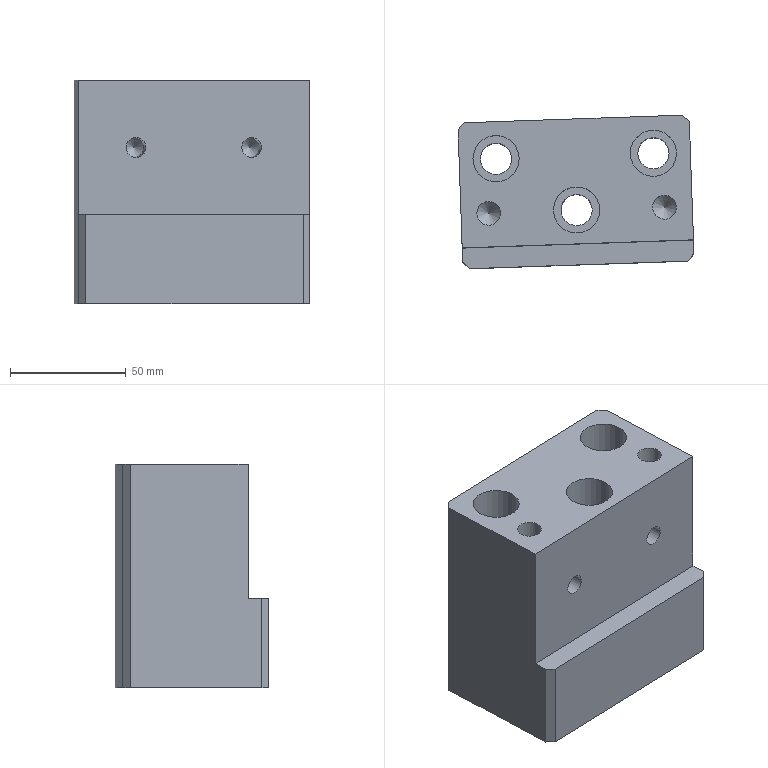Part | NX | features LB-14 2 | 1 solid | 29 faces | box 101.928 x 66.242 x 96.5 mm | volume 491089 mm3 | plane 15 | cylinder 10 | cone 4 | commonest cylinder face diameters 13.5 x3 20 x3 8.506 x2 10.3 x2
STEP:
#1=CARTESIAN_POINT('',(3839.924,-622.872,788.716));
#2=VERTEX_POINT('',#1);
#3=CARTESIAN_POINT('',(3833.174,-622.872,788.716));
#4=DIRECTION('',(-0.000000002,0.,1.));
#5=DIRECTION('',(1.,0.,0.000000002));
#6=AXIS2_PLACEMENT_3D('',#3,#4,#5);
#7=CIRCLE('',#6,6.75);
#8=EDGE_CURVE('',#2,#2,#7,.F.);
#9=ORIENTED_EDGE('',*,*,#8,.F.);
#10=EDGE_LOOP('',(#9));
#11=FACE_BOUND('',#10,.T.);
#12=CARTESIAN_POINT('',(3850.699,-666.287,788.716));
#13=VERTEX_POINT('',#12);
#14=CARTESIAN_POINT('',(3848.71,-609.321,788.716));
#15=VERTEX_POINT('',#14);
#16=CARTESIAN_POINT('',(3848.745,-610.321,788.716));
#17=DIRECTION('',(-0.0349,0.9994,0.));
#18=VECTOR('',#17,1000.);
#19=LINE('',#16,#18);
#20=EDGE_CURVE('',#13,#15,#19,.T.);
#21=ORIENTED_EDGE('',*,*,#20,.F.);
#22=CARTESIAN_POINT('',(3847.806,-669.389,788.716));
#23=VERTEX_POINT('',#22);
#24=CARTESIAN_POINT('',(3830.445,-688.007,788.716));
#25=DIRECTION('',(-0.682,-0.7314,-0.000000001));
#26=VECTOR('',#25,1000.);
#27=LINE('',#24,#26);
#28=EDGE_CURVE('',#23,#13,#27,.F.);
#29=ORIENTED_EDGE('',*,*,#28,.F.);
#30=CARTESIAN_POINT('',(3753.863,-672.67,788.716));
#31=VERTEX_POINT('',#30);
#32=CARTESIAN_POINT('',(3752.864,-672.705,788.716));
#33=DIRECTION('',(0.9994,0.0349,0.000000002));
#34=VECTOR('',#33,1000.);
#35=LINE('',#32,#34);
#36=EDGE_CURVE('',#31,#23,#35,.T.);
#37=ORIENTED_EDGE('',*,*,#36,.F.);
#38=CARTESIAN_POINT('',(3750.76,-669.776,788.716));
#39=VERTEX_POINT('',#38);
#40=CARTESIAN_POINT('',(3722.835,-643.735,788.716));
#41=DIRECTION('',(-0.7314,0.682,-0.000000001));
#42=VECTOR('',#41,1000.);
#43=LINE('',#40,#42);
#44=EDGE_CURVE('',#39,#31,#43,.F.);
#45=ORIENTED_EDGE('',*,*,#44,.F.);
#46=CARTESIAN_POINT('',(3748.771,-612.811,788.716));
#47=VERTEX_POINT('',#46);
#48=CARTESIAN_POINT('',(3748.806,-613.81,788.716));
#49=DIRECTION('',(0.0349,-0.9994,0.));
#50=VECTOR('',#49,1000.);
#51=LINE('',#48,#50);
#52=EDGE_CURVE('',#47,#39,#51,.T.);
#53=ORIENTED_EDGE('',*,*,#52,.F.);
#54=CARTESIAN_POINT('',(3751.665,-609.708,788.716));
#55=VERTEX_POINT('',#54);
#56=CARTESIAN_POINT('',(3749.254,-612.294,788.716));
#57=DIRECTION('',(0.682,0.7314,0.000000001));
#58=VECTOR('',#57,1000.);
#59=LINE('',#56,#58);
#60=EDGE_CURVE('',#55,#47,#59,.F.);
#61=ORIENTED_EDGE('',*,*,#60,.F.);
#62=CARTESIAN_POINT('',(3845.608,-606.428,788.716));
#63=VERTEX_POINT('',#62);
#64=CARTESIAN_POINT('',(3750.665,-609.743,788.716));
#65=DIRECTION('',(-0.9994,-0.0349,-0.000000002));
#66=VECTOR('',#65,1000.);
#67=LINE('',#64,#66);
#68=EDGE_CURVE('',#63,#55,#67,.T.);
#69=ORIENTED_EDGE('',*,*,#68,.F.);
#70=CARTESIAN_POINT('',(3798.548,-562.543,788.716));
#71=DIRECTION('',(0.7314,-0.682,0.000000001));
#72=VECTOR('',#71,1000.);
#73=LINE('',#70,#72);
#74=EDGE_CURVE('',#15,#63,#73,.F.);
#75=ORIENTED_EDGE('',*,*,#74,.F.);
#76=EDGE_LOOP('',(#21,#29,#37,#45,#53,#61,#69,#75));
#77=FACE_BOUND('',#76,.T.);
#78=CARTESIAN_POINT('',(3806.76,-647.401,788.716));
#79=VERTEX_POINT('',#78);
#80=CARTESIAN_POINT('',(3800.01,-647.401,788.716));
#81=DIRECTION('',(-0.000000002,0.,1.));
#82=DIRECTION('',(1.,0.,0.000000002));
#83=AXIS2_PLACEMENT_3D('',#80,#81,#82);
#84=CIRCLE('',#83,6.75);
#85=EDGE_CURVE('',#79,#79,#84,.F.);
#86=ORIENTED_EDGE('',*,*,#85,.F.);
#87=EDGE_LOOP('',(#86));
#88=FACE_BOUND('',#87,.T.);
#89=CARTESIAN_POINT('',(3771.965,-625.245,788.716));
#90=VERTEX_POINT('',#89);
#91=CARTESIAN_POINT('',(3765.215,-625.245,788.716));
#92=DIRECTION('',(-0.000000002,0.,1.));
#93=DIRECTION('',(1.,0.,0.000000002));
#94=AXIS2_PLACEMENT_3D('',#91,#92,#93);
#95=CIRCLE('',#94,6.75);
#96=EDGE_CURVE('',#90,#90,#95,.F.);
#97=ORIENTED_EDGE('',*,*,#96,.F.);
#98=EDGE_LOOP('',(#97));
#99=FACE_BOUND('',#98,.T.);
#100=CARTESIAN_POINT('',(3750.805,-613.741,788.716));
#101=DIRECTION('',(-0.000000002,0.,1.));
#102=DIRECTION('',(0.9994,0.0349,0.000000002));
#103=AXIS2_PLACEMENT_3D('',#100,#101,#102);
#104=PLANE('',#103);
#105=ADVANCED_FACE('',(#11,#77,#88,#99),#104,.F.);
#106=CARTESIAN_POINT('',(3810.01,-647.401,885.216));
#107=VERTEX_POINT('',#106);
#108=CARTESIAN_POINT('',(3800.01,-647.401,885.216));
#109=DIRECTION('',(0.,0.,1.));
#110=DIRECTION('',(1.,0.,0.));
#111=AXIS2_PLACEMENT_3D('',#108,#109,#110);
#112=CIRCLE('',#111,10.);
#113=EDGE_CURVE('',#107,#107,#112,.T.);
#114=ORIENTED_EDGE('',*,*,#113,.F.);
#115=EDGE_LOOP('',(#114));
#116=FACE_BOUND('',#115,.T.);
#117=CARTESIAN_POINT('',(3767.185,-648.69,885.216));
#118=VERTEX_POINT('',#117);
#119=CARTESIAN_POINT('',(3762.038,-648.87,885.216));
#120=DIRECTION('',(0.000000002,0.,-1.));
#121=DIRECTION('',(0.9994,0.0349,0.000000002));
#122=AXIS2_PLACEMENT_3D('',#119,#120,#121);
#123=CIRCLE('',#122,5.15);
#124=EDGE_CURVE('',#118,#118,#123,.T.);
#125=ORIENTED_EDGE('',*,*,#124,.T.);
#126=EDGE_LOOP('',(#125));
#127=FACE_BOUND('',#126,.T.);
#128=CARTESIAN_POINT('',(3843.138,-646.038,885.216));
#129=VERTEX_POINT('',#128);
#130=CARTESIAN_POINT('',(3837.991,-646.218,885.216));
#131=DIRECTION('',(0.000000002,0.,-1.));
#132=DIRECTION('',(0.9994,0.0349,0.000000002));
#133=AXIS2_PLACEMENT_3D('',#130,#131,#132);
#134=CIRCLE('',#133,5.15);
#135=EDGE_CURVE('',#129,#129,#134,.T.);
#136=ORIENTED_EDGE('',*,*,#135,.T.);
#137=EDGE_LOOP('',(#136));
#138=FACE_BOUND('',#137,.T.);
#139=CARTESIAN_POINT('',(3748.771,-612.811,885.216));
#140=VERTEX_POINT('',#139);
#141=CARTESIAN_POINT('',(3750.551,-663.78,885.216));
#142=VERTEX_POINT('',#141);
#143=CARTESIAN_POINT('',(3748.387,-601.818,885.216));
#144=DIRECTION('',(0.0349,-0.9994,0.));
#145=VECTOR('',#144,1000.);
#146=LINE('',#143,#145);
#147=EDGE_CURVE('',#140,#142,#146,.T.);
#148=ORIENTED_EDGE('',*,*,#147,.T.);
#149=CARTESIAN_POINT('',(3850.49,-660.29,885.216));
#150=VERTEX_POINT('',#149);
#151=CARTESIAN_POINT('',(3983.632,-655.641,885.216));
#152=DIRECTION('',(-0.9994,-0.0349,-0.000000002));
#153=VECTOR('',#152,1000.);
#154=LINE('',#151,#153);
#155=EDGE_CURVE('',#150,#142,#154,.T.);
#156=ORIENTED_EDGE('',*,*,#155,.F.);
#157=CARTESIAN_POINT('',(3848.71,-609.321,885.216));
#158=VERTEX_POINT('',#157);
#159=CARTESIAN_POINT('',(3848.745,-610.321,885.216));
#160=DIRECTION('',(0.0349,-0.9994,0.));
#161=VECTOR('',#160,1000.);
#162=LINE('',#159,#161);
#163=EDGE_CURVE('',#158,#150,#162,.T.);
#164=ORIENTED_EDGE('',*,*,#163,.F.);
#165=CARTESIAN_POINT('',(3845.608,-606.428,885.216));
#166=VERTEX_POINT('',#165);
#167=CARTESIAN_POINT('',(3798.548,-562.543,885.216));
#168=DIRECTION('',(-0.7314,0.682,-0.000000001));
#169=VECTOR('',#168,1000.);
#170=LINE('',#167,#169);
#171=EDGE_CURVE('',#166,#158,#170,.F.);
#172=ORIENTED_EDGE('',*,*,#171,.F.);
#173=CARTESIAN_POINT('',(3751.665,-609.708,885.216));
#174=VERTEX_POINT('',#173);
#175=CARTESIAN_POINT('',(3813.627,-607.545,885.216));
#176=DIRECTION('',(-0.9994,-0.0349,-0.000000002));
#177=VECTOR('',#176,1000.);
#178=LINE('',#175,#177);
#179=EDGE_CURVE('',#166,#174,#178,.T.);
#180=ORIENTED_EDGE('',*,*,#179,.T.);
#181=CARTESIAN_POINT('',(3749.254,-612.294,885.216));
#182=DIRECTION('',(-0.682,-0.7314,-0.000000001));
#183=VECTOR('',#182,1000.);
#184=LINE('',#181,#183);
#185=EDGE_CURVE('',#140,#174,#184,.F.);
#186=ORIENTED_EDGE('',*,*,#185,.F.);
#187=EDGE_LOOP('',(#148,#156,#164,#172,#180,#186));
#188=FACE_BOUND('',#187,.T.);
#189=CARTESIAN_POINT('',(3775.215,-625.245,885.216));
#190=VERTEX_POINT('',#189);
#191=CARTESIAN_POINT('',(3765.215,-625.245,885.216));
#192=DIRECTION('',(0.,0.,1.));
#193=DIRECTION('',(1.,0.,0.));
#194=AXIS2_PLACEMENT_3D('',#191,#192,#193);
#195=CIRCLE('',#194,10.);
#196=EDGE_CURVE('',#190,#190,#195,.T.);
#197=ORIENTED_EDGE('',*,*,#196,.F.);
#198=EDGE_LOOP('',(#197));
#199=FACE_BOUND('',#198,.T.);
#200=CARTESIAN_POINT('',(3843.174,-622.872,885.216));
#201=VERTEX_POINT('',#200);
#202=CARTESIAN_POINT('',(3833.174,-622.872,885.216));
#203=DIRECTION('',(0.,0.,1.));
#204=DIRECTION('',(1.,0.,0.));
#205=AXIS2_PLACEMENT_3D('',#202,#203,#204);
#206=CIRCLE('',#205,10.);
#207=EDGE_CURVE('',#201,#201,#206,.T.);
#208=ORIENTED_EDGE('',*,*,#207,.F.);
#209=EDGE_LOOP('',(#208));
#210=FACE_BOUND('',#209,.T.);
#211=CARTESIAN_POINT('',(3750.805,-613.741,885.216));
#212=DIRECTION('',(-0.000000002,0.,1.));
#213=DIRECTION('',(0.9994,0.0349,0.000000002));
#214=AXIS2_PLACEMENT_3D('',#211,#212,#213);
#215=PLANE('',#214);
#216=ADVANCED_FACE('',(#116,#127,#138,#188,#199,#210),#215,.T.);
#217=CARTESIAN_POINT('',(3775.536,-662.907,851.963));
#218=VERTEX_POINT('',#217);
#219=CARTESIAN_POINT('',(3775.536,-662.907,856.216));
#220=DIRECTION('',(0.0349,-0.9994,0.));
#221=DIRECTION('',(0.000000002,0.,-1.));
#222=AXIS2_PLACEMENT_3D('',#219,#220,#221);
#223=CIRCLE('',#222,4.253);
#224=EDGE_CURVE('',#218,#218,#223,.T.);
#225=ORIENTED_EDGE('',*,*,#224,.T.);
#226=EDGE_LOOP('',(#225));
#227=FACE_BOUND('',#226,.T.);
#228=CARTESIAN_POINT('',(3774.637,-637.176,860.469));
#229=VERTEX_POINT('',#228);
#230=CARTESIAN_POINT('',(3774.637,-637.176,856.216));
#231=DIRECTION('',(-0.0349,0.9994,0.));
#232=DIRECTION('',(-0.000000002,0.,1.));
#233=AXIS2_PLACEMENT_3D('',#230,#231,#232);
#234=CIRCLE('',#233,4.253);
#235=EDGE_CURVE('',#229,#229,#234,.F.);
#236=ORIENTED_EDGE('',*,*,#235,.F.);
#237=EDGE_LOOP('',(#236));
#238=FACE_BOUND('',#237,.T.);
#239=CARTESIAN_POINT('',(3775.536,-662.907,856.216));
#240=DIRECTION('',(-0.0349,0.9994,0.));
#241=DIRECTION('',(-0.9994,-0.0349,-0.000000002));
#242=AXIS2_PLACEMENT_3D('',#239,#240,#241);
#243=CYLINDRICAL_SURFACE('',#242,4.253);
#244=ADVANCED_FACE('',(#227,#238),#243,.F.);
#245=CARTESIAN_POINT('',(3825.505,-661.163,851.963));
#246=VERTEX_POINT('',#245);
#247=CARTESIAN_POINT('',(3825.505,-661.163,856.216));
#248=DIRECTION('',(0.0349,-0.9994,0.));
#249=DIRECTION('',(0.000000002,0.,-1.));
#250=AXIS2_PLACEMENT_3D('',#247,#248,#249);
#251=CIRCLE('',#250,4.253);
#252=EDGE_CURVE('',#246,#246,#251,.T.);
#253=ORIENTED_EDGE('',*,*,#252,.T.);
#254=EDGE_LOOP('',(#253));
#255=FACE_BOUND('',#254,.T.);
#256=CARTESIAN_POINT('',(3824.607,-635.431,860.469));
#257=VERTEX_POINT('',#256);
#258=CARTESIAN_POINT('',(3824.607,-635.431,856.216));
#259=DIRECTION('',(-0.0349,0.9994,0.));
#260=DIRECTION('',(-0.000000002,0.,1.));
#261=AXIS2_PLACEMENT_3D('',#258,#259,#260);
#262=CIRCLE('',#261,4.253);
#263=EDGE_CURVE('',#257,#257,#262,.F.);
#264=ORIENTED_EDGE('',*,*,#263,.F.);
#265=EDGE_LOOP('',(#264));
#266=FACE_BOUND('',#265,.T.);
#267=CARTESIAN_POINT('',(3825.505,-661.163,856.216));
#268=DIRECTION('',(-0.0349,0.9994,0.));
#269=DIRECTION('',(-0.9994,-0.0349,-0.000000002));
#270=AXIS2_PLACEMENT_3D('',#267,#268,#269);
#271=CYLINDRICAL_SURFACE('',#270,4.253);
#272=ADVANCED_FACE('',(#255,#266),#271,.F.);
#273=CARTESIAN_POINT('',(3848.71,-609.321,814.439));
#274=DIRECTION('',(0.000000002,0.,-1.));
#275=VECTOR('',#274,1000.);
#276=LINE('',#273,#275);
#277=EDGE_CURVE('',#158,#15,#276,.T.);
#278=ORIENTED_EDGE('',*,*,#277,.F.);
#279=ORIENTED_EDGE('',*,*,#163,.T.);
#280=CARTESIAN_POINT('',(3850.49,-660.29,827.216));
#281=VERTEX_POINT('',#280);
#282=CARTESIAN_POINT('',(3850.49,-660.29,814.439));
#283=DIRECTION('',(0.000000002,0.,-1.));
#284=VECTOR('',#283,1000.);
#285=LINE('',#282,#284);
#286=EDGE_CURVE('',#150,#281,#285,.T.);
#287=ORIENTED_EDGE('',*,*,#286,.T.);
#288=CARTESIAN_POINT('',(3850.699,-666.287,827.216));
#289=VERTEX_POINT('',#288);
#290=CARTESIAN_POINT('',(3858.049,-876.766,827.216));
#291=DIRECTION('',(0.0349,-0.9994,0.));
#292=VECTOR('',#291,1000.);
#293=LINE('',#290,#292);
#294=EDGE_CURVE('',#281,#289,#293,.T.);
#295=ORIENTED_EDGE('',*,*,#294,.T.);
#296=CARTESIAN_POINT('',(3850.699,-666.287,814.439));
#297=DIRECTION('',(0.000000002,0.,-1.));
#298=VECTOR('',#297,1000.);
#299=LINE('',#296,#298);
#300=EDGE_CURVE('',#13,#289,#299,.F.);
#301=ORIENTED_EDGE('',*,*,#300,.F.);
#302=ORIENTED_EDGE('',*,*,#20,.T.);
#303=EDGE_LOOP('',(#278,#279,#287,#295,#301,#302));
#304=FACE_BOUND('',#303,.T.);
#305=CARTESIAN_POINT('',(3858.049,-876.766,814.439));
#306=DIRECTION('',(0.9994,0.0349,0.000000002));
#307=DIRECTION('',(0.000000002,0.,-1.));
#308=AXIS2_PLACEMENT_3D('',#305,#306,#307);
#309=PLANE('',#308);
#310=ADVANCED_FACE('',(#304),#309,.T.);
#311=ORIENTED_EDGE('',*,*,#52,.T.);
#312=CARTESIAN_POINT('',(3750.76,-669.776,827.216));
#313=VERTEX_POINT('',#312);
#314=CARTESIAN_POINT('',(3750.76,-669.776,851.216));
#315=DIRECTION('',(-0.000000002,0.,1.));
#316=VECTOR('',#315,1000.);
#317=LINE('',#314,#316);
#318=EDGE_CURVE('',#313,#39,#317,.F.);
#319=ORIENTED_EDGE('',*,*,#318,.F.);
#320=CARTESIAN_POINT('',(3750.551,-663.78,827.216));
#321=VERTEX_POINT('',#320);
#322=CARTESIAN_POINT('',(3748.387,-601.818,827.216));
#323=DIRECTION('',(-0.0349,0.9994,0.));
#324=VECTOR('',#323,1000.);
#325=LINE('',#322,#324);
#326=EDGE_CURVE('',#313,#321,#325,.T.);
#327=ORIENTED_EDGE('',*,*,#326,.T.);
#328=CARTESIAN_POINT('',(3750.551,-663.78,851.216));
#329=DIRECTION('',(-0.000000002,0.,1.));
#330=VECTOR('',#329,1000.);
#331=LINE('',#328,#330);
#332=EDGE_CURVE('',#321,#142,#331,.T.);
#333=ORIENTED_EDGE('',*,*,#332,.T.);
#334=ORIENTED_EDGE('',*,*,#147,.F.);
#335=CARTESIAN_POINT('',(3748.771,-612.811,851.216));
#336=DIRECTION('',(-0.000000002,0.,1.));
#337=VECTOR('',#336,1000.);
#338=LINE('',#335,#337);
#339=EDGE_CURVE('',#47,#140,#338,.T.);
#340=ORIENTED_EDGE('',*,*,#339,.F.);
#341=EDGE_LOOP('',(#311,#319,#327,#333,#334,#340));
#342=FACE_BOUND('',#341,.T.);
#343=CARTESIAN_POINT('',(3748.387,-601.818,851.216));
#344=DIRECTION('',(-0.9994,-0.0349,-0.000000002));
#345=DIRECTION('',(-0.000000002,0.,1.));
#346=AXIS2_PLACEMENT_3D('',#343,#344,#345);
#347=PLANE('',#346);
#348=ADVANCED_FACE('',(#342),#347,.T.);
#349=CARTESIAN_POINT('',(3793.26,-647.401,860.216));
#350=VERTEX_POINT('',#349);
#351=CARTESIAN_POINT('',(3800.01,-647.401,860.216));
#352=DIRECTION('',(0.,0.,1.));
#353=DIRECTION('',(-1.,0.,0.));
#354=AXIS2_PLACEMENT_3D('',#351,#352,#353);
#355=CIRCLE('',#354,6.75);
#356=EDGE_CURVE('',#350,#350,#355,.T.);
#357=ORIENTED_EDGE('',*,*,#356,.F.);
#358=EDGE_LOOP('',(#357));
#359=FACE_BOUND('',#358,.T.);
#360=CARTESIAN_POINT('',(3810.01,-647.401,860.216));
#361=VERTEX_POINT('',#360);
#362=CARTESIAN_POINT('',(3800.01,-647.401,860.216));
#363=DIRECTION('',(0.,0.,-1.));
#364=DIRECTION('',(1.,0.,0.));
#365=AXIS2_PLACEMENT_3D('',#362,#363,#364);
#366=CIRCLE('',#365,10.);
#367=EDGE_CURVE('',#361,#361,#366,.F.);
#368=ORIENTED_EDGE('',*,*,#367,.T.);
#369=EDGE_LOOP('',(#368));
#370=FACE_BOUND('',#369,.T.);
#371=CARTESIAN_POINT('',(3800.01,-647.401,860.216));
#372=DIRECTION('',(0.,0.,-1.));
#373=DIRECTION('',(-1.,0.,0.));
#374=AXIS2_PLACEMENT_3D('',#371,#372,#373);
#375=PLANE('',#374);
#376=ADVANCED_FACE('',(#359,#370),#375,.F.);
#377=ORIENTED_EDGE('',*,*,#113,.T.);
#378=EDGE_LOOP('',(#377));
#379=FACE_BOUND('',#378,.T.);
#380=ORIENTED_EDGE('',*,*,#367,.F.);
#381=EDGE_LOOP('',(#380));
#382=FACE_BOUND('',#381,.T.);
#383=CARTESIAN_POINT('',(3800.01,-647.401,885.216));
#384=DIRECTION('',(0.,0.,-1.));
#385=DIRECTION('',(1.,0.,0.));
#386=AXIS2_PLACEMENT_3D('',#383,#384,#385);
#387=CYLINDRICAL_SURFACE('',#386,10.);
#388=ADVANCED_FACE('',(#379,#382),#387,.F.);
#389=CARTESIAN_POINT('',(3837.991,-646.218,845.216));
#390=VERTEX_POINT('',#389);
#391=VERTEX_LOOP('',#390);
#392=FACE_BOUND('',#391,.T.);
#393=CARTESIAN_POINT('',(3843.138,-646.038,850.366));
#394=VERTEX_POINT('',#393);
#395=CARTESIAN_POINT('',(3837.991,-646.218,850.366));
#396=DIRECTION('',(0.000000002,0.,-1.));
#397=DIRECTION('',(0.9994,0.0349,0.000000002));
#398=AXIS2_PLACEMENT_3D('',#395,#396,#397);
#399=CIRCLE('',#398,5.15);
#400=EDGE_CURVE('',#394,#394,#399,.T.);
#401=ORIENTED_EDGE('',*,*,#400,.F.);
#402=EDGE_LOOP('',(#401));
#403=FACE_BOUND('',#402,.T.);
#404=CARTESIAN_POINT('',(3837.991,-646.218,850.466));
#405=DIRECTION('',(-0.000000002,0.,1.));
#406=DIRECTION('',(-0.9994,-0.0349,-0.000000002));
#407=AXIS2_PLACEMENT_3D('',#404,#405,#406);
#408=CONICAL_SURFACE('',#407,5.25,0.7854);
#409=ADVANCED_FACE('',(#392,#403),#408,.F.);
#410=CARTESIAN_POINT('',(3762.038,-648.87,845.216));
#411=VERTEX_POINT('',#410);
#412=VERTEX_LOOP('',#411);
#413=FACE_BOUND('',#412,.T.);
#414=CARTESIAN_POINT('',(3767.185,-648.69,850.366));
#415=VERTEX_POINT('',#414);
#416=CARTESIAN_POINT('',(3762.038,-648.87,850.366));
#417=DIRECTION('',(0.000000002,0.,-1.));
#418=DIRECTION('',(0.9994,0.0349,0.000000002));
#419=AXIS2_PLACEMENT_3D('',#416,#417,#418);
#420=CIRCLE('',#419,5.15);
#421=EDGE_CURVE('',#415,#415,#420,.F.);
#422=ORIENTED_EDGE('',*,*,#421,.T.);
#423=EDGE_LOOP('',(#422));
#424=FACE_BOUND('',#423,.T.);
#425=CARTESIAN_POINT('',(3762.038,-648.87,850.466));
#426=DIRECTION('',(-0.000000002,0.,1.));
#427=DIRECTION('',(0.9994,0.0349,0.000000002));
#428=AXIS2_PLACEMENT_3D('',#425,#426,#427);
#429=CONICAL_SURFACE('',#428,5.25,0.7854);
#430=ADVANCED_FACE('',(#413,#424),#429,.F.);
#431=ORIENTED_EDGE('',*,*,#294,.F.);
#432=CARTESIAN_POINT('',(3983.632,-655.641,827.216));
#433=DIRECTION('',(-0.9994,-0.0349,-0.000000002));
#434=VECTOR('',#433,1000.);
#435=LINE('',#432,#434);
#436=EDGE_CURVE('',#281,#321,#435,.T.);
#437=ORIENTED_EDGE('',*,*,#436,.T.);
#438=ORIENTED_EDGE('',*,*,#326,.F.);
#439=CARTESIAN_POINT('',(3753.863,-672.67,827.216));
#440=VERTEX_POINT('',#439);
#441=CARTESIAN_POINT('',(3753.863,-672.67,827.216));
#442=DIRECTION('',(0.7314,-0.682,0.000000001));
#443=VECTOR('',#442,1000.);
#444=LINE('',#441,#443);
#445=EDGE_CURVE('',#440,#313,#444,.F.);
#446=ORIENTED_EDGE('',*,*,#445,.F.);
#447=CARTESIAN_POINT('',(3847.806,-669.389,827.216));
#448=VERTEX_POINT('',#447);
#449=CARTESIAN_POINT('',(3740.871,-673.123,827.216));
#450=DIRECTION('',(-0.9994,-0.0349,-0.000000002));
#451=VECTOR('',#450,1000.);
#452=LINE('',#449,#451);
#453=EDGE_CURVE('',#448,#440,#452,.T.);
#454=ORIENTED_EDGE('',*,*,#453,.F.);
#455=CARTESIAN_POINT('',(3855.522,-661.115,827.216));
#456=DIRECTION('',(0.682,0.7314,0.000000001));
#457=VECTOR('',#456,1000.);
#458=LINE('',#455,#457);
#459=EDGE_CURVE('',#289,#448,#458,.F.);
#460=ORIENTED_EDGE('',*,*,#459,.F.);
#461=EDGE_LOOP('',(#431,#437,#438,#446,#454,#460));
#462=FACE_BOUND('',#461,.T.);
#463=CARTESIAN_POINT('',(3983.946,-664.636,827.216));
#464=DIRECTION('',(0.000000002,0.,-1.));
#465=DIRECTION('',(-0.9994,-0.0349,-0.000000002));
#466=AXIS2_PLACEMENT_3D('',#463,#464,#465);
#467=PLANE('',#466);
#468=ADVANCED_FACE('',(#462),#467,.F.);
#469=ORIENTED_EDGE('',*,*,#252,.F.);
#470=EDGE_LOOP('',(#469));
#471=FACE_BOUND('',#470,.T.);
#472=ORIENTED_EDGE('',*,*,#224,.F.);
#473=EDGE_LOOP('',(#472));
#474=FACE_BOUND('',#473,.T.);
#475=ORIENTED_EDGE('',*,*,#286,.F.);
#476=ORIENTED_EDGE('',*,*,#155,.T.);
#477=ORIENTED_EDGE('',*,*,#332,.F.);
#478=ORIENTED_EDGE('',*,*,#436,.F.);
#479=EDGE_LOOP('',(#475,#476,#477,#478));
#480=FACE_BOUND('',#479,.T.);
#481=CARTESIAN_POINT('',(3983.632,-655.641,833.216));
#482=DIRECTION('',(-0.0349,0.9994,0.));
#483=DIRECTION('',(0.000000002,0.,-1.));
#484=AXIS2_PLACEMENT_3D('',#481,#482,#483);
#485=PLANE('',#484);
#486=ADVANCED_FACE('',(#471,#474,#480),#485,.F.);
#487=ORIENTED_EDGE('',*,*,#453,.T.);
#488=CARTESIAN_POINT('',(3753.863,-672.67,851.216));
#489=DIRECTION('',(-0.000000002,0.,1.));
#490=VECTOR('',#489,1000.);
#491=LINE('',#488,#490);
#492=EDGE_CURVE('',#31,#440,#491,.T.);
#493=ORIENTED_EDGE('',*,*,#492,.F.);
#494=ORIENTED_EDGE('',*,*,#36,.T.);
#495=CARTESIAN_POINT('',(3847.806,-669.389,851.216));
#496=DIRECTION('',(0.000000002,0.,-1.));
#497=VECTOR('',#496,1000.);
#498=LINE('',#495,#497);
#499=EDGE_CURVE('',#448,#23,#498,.T.);
#500=ORIENTED_EDGE('',*,*,#499,.F.);
#501=EDGE_LOOP('',(#487,#493,#494,#500));
#502=FACE_BOUND('',#501,.T.);
#503=CARTESIAN_POINT('',(3740.871,-673.123,851.216));
#504=DIRECTION('',(0.0349,-0.9994,0.));
#505=DIRECTION('',(-0.000000002,0.,1.));
#506=AXIS2_PLACEMENT_3D('',#503,#504,#505);
#507=PLANE('',#506);
#508=ADVANCED_FACE('',(#502),#507,.T.);
#509=ORIENTED_EDGE('',*,*,#135,.F.);
#510=EDGE_LOOP('',(#509));
#511=FACE_BOUND('',#510,.T.);
#512=ORIENTED_EDGE('',*,*,#400,.T.);
#513=EDGE_LOOP('',(#512));
#514=FACE_BOUND('',#513,.T.);
#515=CARTESIAN_POINT('',(3837.991,-646.218,895.216));
#516=DIRECTION('',(0.000000002,0.,-1.));
#517=DIRECTION('',(0.9994,0.0349,0.000000002));
#518=AXIS2_PLACEMENT_3D('',#515,#516,#517);
#519=CYLINDRICAL_SURFACE('',#518,5.15);
#520=ADVANCED_FACE('',(#511,#514),#519,.F.);
#521=ORIENTED_EDGE('',*,*,#124,.F.);
#522=EDGE_LOOP('',(#521));
#523=FACE_BOUND('',#522,.T.);
#524=ORIENTED_EDGE('',*,*,#421,.F.);
#525=EDGE_LOOP('',(#524));
#526=FACE_BOUND('',#525,.T.);
#527=CARTESIAN_POINT('',(3762.038,-648.87,895.216));
#528=DIRECTION('',(0.000000002,0.,-1.));
#529=DIRECTION('',(-0.9994,-0.0349,-0.000000002));
#530=AXIS2_PLACEMENT_3D('',#527,#528,#529);
#531=CYLINDRICAL_SURFACE('',#530,5.15);
#532=ADVANCED_FACE('',(#523,#526),#531,.F.);
#533=ORIENTED_EDGE('',*,*,#28,.T.);
#534=ORIENTED_EDGE('',*,*,#300,.T.);
#535=ORIENTED_EDGE('',*,*,#459,.T.);
#536=ORIENTED_EDGE('',*,*,#499,.T.);
#537=EDGE_LOOP('',(#533,#534,#535,#536));
#538=FACE_BOUND('',#537,.T.);
#539=CARTESIAN_POINT('',(3855.522,-661.115,814.439));
#540=DIRECTION('',(-0.7314,0.682,-0.000000001));
#541=DIRECTION('',(-0.000000002,0.,1.));
#542=AXIS2_PLACEMENT_3D('',#539,#540,#541);
#543=PLANE('',#542);
#544=ADVANCED_FACE('',(#538),#543,.F.);
#545=ORIENTED_EDGE('',*,*,#44,.T.);
#546=ORIENTED_EDGE('',*,*,#492,.T.);
#547=ORIENTED_EDGE('',*,*,#445,.T.);
#548=ORIENTED_EDGE('',*,*,#318,.T.);
#549=EDGE_LOOP('',(#545,#546,#547,#548));
#550=FACE_BOUND('',#549,.T.);
#551=CARTESIAN_POINT('',(3753.863,-672.67,851.216));
#552=DIRECTION('',(0.682,0.7314,0.000000001));
#553=DIRECTION('',(-0.000000002,0.,1.));
#554=AXIS2_PLACEMENT_3D('',#551,#552,#553);
#555=PLANE('',#554);
#556=ADVANCED_FACE('',(#550),#555,.F.);
#557=ORIENTED_EDGE('',*,*,#356,.T.);
#558=EDGE_LOOP('',(#557));
#559=FACE_BOUND('',#558,.T.);
#560=ORIENTED_EDGE('',*,*,#85,.T.);
#561=EDGE_LOOP('',(#560));
#562=FACE_BOUND('',#561,.T.);
#563=CARTESIAN_POINT('',(3800.01,-647.401,885.216));
#564=DIRECTION('',(0.,0.,-1.));
#565=DIRECTION('',(1.,0.,0.));
#566=AXIS2_PLACEMENT_3D('',#563,#564,#565);
#567=CYLINDRICAL_SURFACE('',#566,6.75);
#568=ADVANCED_FACE('',(#559,#562),#567,.F.);
#569=ORIENTED_EDGE('',*,*,#235,.T.);
#570=EDGE_LOOP('',(#569));
#571=FACE_BOUND('',#570,.T.);
#572=CARTESIAN_POINT('',(3774.489,-632.926,856.216));
#573=VERTEX_POINT('',#572);
#574=VERTEX_LOOP('',#573);
#575=FACE_BOUND('',#574,.T.);
#576=CARTESIAN_POINT('',(3774.637,-637.173,856.216));
#577=DIRECTION('',(0.0349,-0.9994,0.));
#578=DIRECTION('',(-0.000000002,0.,1.));
#579=AXIS2_PLACEMENT_3D('',#576,#577,#578);
#580=CONICAL_SURFACE('',#579,4.25,0.7854);
#581=ADVANCED_FACE('',(#571,#575),#580,.F.);
#582=ORIENTED_EDGE('',*,*,#263,.T.);
#583=EDGE_LOOP('',(#582));
#584=FACE_BOUND('',#583,.T.);
#585=CARTESIAN_POINT('',(3824.458,-631.181,856.216));
#586=VERTEX_POINT('',#585);
#587=VERTEX_LOOP('',#586);
#588=FACE_BOUND('',#587,.T.);
#589=CARTESIAN_POINT('',(3824.607,-635.428,856.216));
#590=DIRECTION('',(0.0349,-0.9994,0.));
#591=DIRECTION('',(-0.000000002,0.,1.));
#592=AXIS2_PLACEMENT_3D('',#589,#590,#591);
#593=CONICAL_SURFACE('',#592,4.25,0.7854);
#594=ADVANCED_FACE('',(#584,#588),#593,.F.);
#595=CARTESIAN_POINT('',(3826.424,-622.872,860.216));
#596=VERTEX_POINT('',#595);
#597=CARTESIAN_POINT('',(3833.174,-622.872,860.216));
#598=DIRECTION('',(0.,0.,1.));
#599=DIRECTION('',(-1.,0.,0.));
#600=AXIS2_PLACEMENT_3D('',#597,#598,#599);
#601=CIRCLE('',#600,6.75);
#602=EDGE_CURVE('',#596,#596,#601,.T.);
#603=ORIENTED_EDGE('',*,*,#602,.T.);
#604=EDGE_LOOP('',(#603));
#605=FACE_BOUND('',#604,.T.);
#606=ORIENTED_EDGE('',*,*,#8,.T.);
#607=EDGE_LOOP('',(#606));
#608=FACE_BOUND('',#607,.T.);
#609=CARTESIAN_POINT('',(3833.174,-622.872,885.216));
#610=DIRECTION('',(0.,0.,-1.));
#611=DIRECTION('',(1.,0.,0.));
#612=AXIS2_PLACEMENT_3D('',#609,#610,#611);
#613=CYLINDRICAL_SURFACE('',#612,6.75);
#614=ADVANCED_FACE('',(#605,#608),#613,.F.);
#615=CARTESIAN_POINT('',(3758.465,-625.245,860.216));
#616=VERTEX_POINT('',#615);
#617=CARTESIAN_POINT('',(3765.215,-625.245,860.216));
#618=DIRECTION('',(0.,0.,1.));
#619=DIRECTION('',(-1.,0.,0.));
#620=AXIS2_PLACEMENT_3D('',#617,#618,#619);
#621=CIRCLE('',#620,6.75);
#622=EDGE_CURVE('',#616,#616,#621,.T.);
#623=ORIENTED_EDGE('',*,*,#622,.T.);
#624=EDGE_LOOP('',(#623));
#625=FACE_BOUND('',#624,.T.);
#626=ORIENTED_EDGE('',*,*,#96,.T.);
#627=EDGE_LOOP('',(#626));
#628=FACE_BOUND('',#627,.T.);
#629=CARTESIAN_POINT('',(3765.215,-625.245,885.216));
#630=DIRECTION('',(0.,0.,-1.));
#631=DIRECTION('',(1.,0.,0.));
#632=AXIS2_PLACEMENT_3D('',#629,#630,#631);
#633=CYLINDRICAL_SURFACE('',#632,6.75);
#634=ADVANCED_FACE('',(#625,#628),#633,.F.);
#635=ORIENTED_EDGE('',*,*,#171,.T.);
#636=ORIENTED_EDGE('',*,*,#277,.T.);
#637=ORIENTED_EDGE('',*,*,#74,.T.);
#638=CARTESIAN_POINT('',(3845.608,-606.428,851.216));
#639=DIRECTION('',(-0.000000002,0.,1.));
#640=VECTOR('',#639,1000.);
#641=LINE('',#638,#640);
#642=EDGE_CURVE('',#63,#166,#641,.T.);
#643=ORIENTED_EDGE('',*,*,#642,.T.);
#644=EDGE_LOOP('',(#635,#636,#637,#643));
#645=FACE_BOUND('',#644,.T.);
#646=CARTESIAN_POINT('',(3848.71,-609.321,814.439));
#647=DIRECTION('',(-0.682,-0.7314,-0.000000001));
#648=DIRECTION('',(0.000000002,0.,-1.));
#649=AXIS2_PLACEMENT_3D('',#646,#647,#648);
#650=PLANE('',#649);
#651=ADVANCED_FACE('',(#645),#650,.F.);
#652=CARTESIAN_POINT('',(3751.665,-609.708,851.216));
#653=DIRECTION('',(0.000000002,0.,-1.));
#654=VECTOR('',#653,1000.);
#655=LINE('',#652,#654);
#656=EDGE_CURVE('',#174,#55,#655,.T.);
#657=ORIENTED_EDGE('',*,*,#656,.F.);
#658=ORIENTED_EDGE('',*,*,#179,.F.);
#659=ORIENTED_EDGE('',*,*,#642,.F.);
#660=ORIENTED_EDGE('',*,*,#68,.T.);
#661=EDGE_LOOP('',(#657,#658,#659,#660));
#662=FACE_BOUND('',#661,.T.);
#663=CARTESIAN_POINT('',(3813.627,-607.545,851.216));
#664=DIRECTION('',(-0.0349,0.9994,0.));
#665=DIRECTION('',(0.000000002,0.,-1.));
#666=AXIS2_PLACEMENT_3D('',#663,#664,#665);
#667=PLANE('',#666);
#668=ADVANCED_FACE('',(#662),#667,.T.);
#669=ORIENTED_EDGE('',*,*,#185,.T.);
#670=ORIENTED_EDGE('',*,*,#656,.T.);
#671=ORIENTED_EDGE('',*,*,#60,.T.);
#672=ORIENTED_EDGE('',*,*,#339,.T.);
#673=EDGE_LOOP('',(#669,#670,#671,#672));
#674=FACE_BOUND('',#673,.T.);
#675=CARTESIAN_POINT('',(3751.665,-609.708,851.216));
#676=DIRECTION('',(0.7314,-0.682,0.000000001));
#677=DIRECTION('',(0.000000002,0.,-1.));
#678=AXIS2_PLACEMENT_3D('',#675,#676,#677);
#679=PLANE('',#678);
#680=ADVANCED_FACE('',(#674),#679,.F.);
#681=CARTESIAN_POINT('',(3775.215,-625.245,860.216));
#682=VERTEX_POINT('',#681);
#683=CARTESIAN_POINT('',(3765.215,-625.245,860.216));
#684=DIRECTION('',(0.,0.,-1.));
#685=DIRECTION('',(1.,0.,0.));
#686=AXIS2_PLACEMENT_3D('',#683,#684,#685);
#687=CIRCLE('',#686,10.);
#688=EDGE_CURVE('',#682,#682,#687,.F.);
#689=ORIENTED_EDGE('',*,*,#688,.F.);
#690=EDGE_LOOP('',(#689));
#691=FACE_BOUND('',#690,.T.);
#692=ORIENTED_EDGE('',*,*,#196,.T.);
#693=EDGE_LOOP('',(#692));
#694=FACE_BOUND('',#693,.T.);
#695=CARTESIAN_POINT('',(3765.215,-625.245,885.216));
#696=DIRECTION('',(0.,0.,-1.));
#697=DIRECTION('',(1.,0.,0.));
#698=AXIS2_PLACEMENT_3D('',#695,#696,#697);
#699=CYLINDRICAL_SURFACE('',#698,10.);
#700=ADVANCED_FACE('',(#691,#694),#699,.F.);
#701=CARTESIAN_POINT('',(3843.174,-622.872,860.216));
#702=VERTEX_POINT('',#701);
#703=CARTESIAN_POINT('',(3833.174,-622.872,860.216));
#704=DIRECTION('',(0.,0.,-1.));
#705=DIRECTION('',(1.,0.,0.));
#706=AXIS2_PLACEMENT_3D('',#703,#704,#705);
#707=CIRCLE('',#706,10.);
#708=EDGE_CURVE('',#702,#702,#707,.F.);
#709=ORIENTED_EDGE('',*,*,#708,.F.);
#710=EDGE_LOOP('',(#709));
#711=FACE_BOUND('',#710,.T.);
#712=ORIENTED_EDGE('',*,*,#207,.T.);
#713=EDGE_LOOP('',(#712));
#714=FACE_BOUND('',#713,.T.);
#715=CARTESIAN_POINT('',(3833.174,-622.872,885.216));
#716=DIRECTION('',(0.,0.,-1.));
#717=DIRECTION('',(1.,0.,0.));
#718=AXIS2_PLACEMENT_3D('',#715,#716,#717);
#719=CYLINDRICAL_SURFACE('',#718,10.);
#720=ADVANCED_FACE('',(#711,#714),#719,.F.);
#721=ORIENTED_EDGE('',*,*,#602,.F.);
#722=EDGE_LOOP('',(#721));
#723=FACE_BOUND('',#722,.T.);
#724=ORIENTED_EDGE('',*,*,#708,.T.);
#725=EDGE_LOOP('',(#724));
#726=FACE_BOUND('',#725,.T.);
#727=CARTESIAN_POINT('',(3833.174,-622.872,860.216));
#728=DIRECTION('',(0.,0.,-1.));
#729=DIRECTION('',(-1.,0.,0.));
#730=AXIS2_PLACEMENT_3D('',#727,#728,#729);
#731=PLANE('',#730);
#732=ADVANCED_FACE('',(#723,#726),#731,.F.);
#733=ORIENTED_EDGE('',*,*,#622,.F.);
#734=EDGE_LOOP('',(#733));
#735=FACE_BOUND('',#734,.T.);
#736=ORIENTED_EDGE('',*,*,#688,.T.);
#737=EDGE_LOOP('',(#736));
#738=FACE_BOUND('',#737,.T.);
#739=CARTESIAN_POINT('',(3765.215,-625.245,860.216));
#740=DIRECTION('',(0.,0.,-1.));
#741=DIRECTION('',(-1.,0.,0.));
#742=AXIS2_PLACEMENT_3D('',#739,#740,#741);
#743=PLANE('',#742);
#744=ADVANCED_FACE('',(#735,#738),#743,.F.);
#745=CLOSED_SHELL('',(#105,#216,#244,#272,#310,#348,#376,#388,#409,#430,#468,#486,#508,#520,#532,#544,#556,#568,#581,#594,#614,#634,#651,#668,#680,#700,#720,#732,#744));
#746=MANIFOLD_SOLID_BREP('',#745);
#747=(LENGTH_UNIT()NAMED_UNIT(*)SI_UNIT(.MILLI.,.METRE.));
#748=UNCERTAINTY_MEASURE_WITH_UNIT(LENGTH_MEASURE(0.00001),#747,'','');
#749=(NAMED_UNIT(*)PLANE_ANGLE_UNIT()SI_UNIT($,.RADIAN.));
#750=(NAMED_UNIT(*)SI_UNIT($,.STERADIAN.)SOLID_ANGLE_UNIT());
#751=(GEOMETRIC_REPRESENTATION_CONTEXT(3)GLOBAL_UNCERTAINTY_ASSIGNED_CONTEXT((#748))GLOBAL_UNIT_ASSIGNED_CONTEXT((#747,#749,#750))REPRESENTATION_CONTEXT('',''));
#752=ADVANCED_BREP_SHAPE_REPRESENTATION('',(#746),#751);